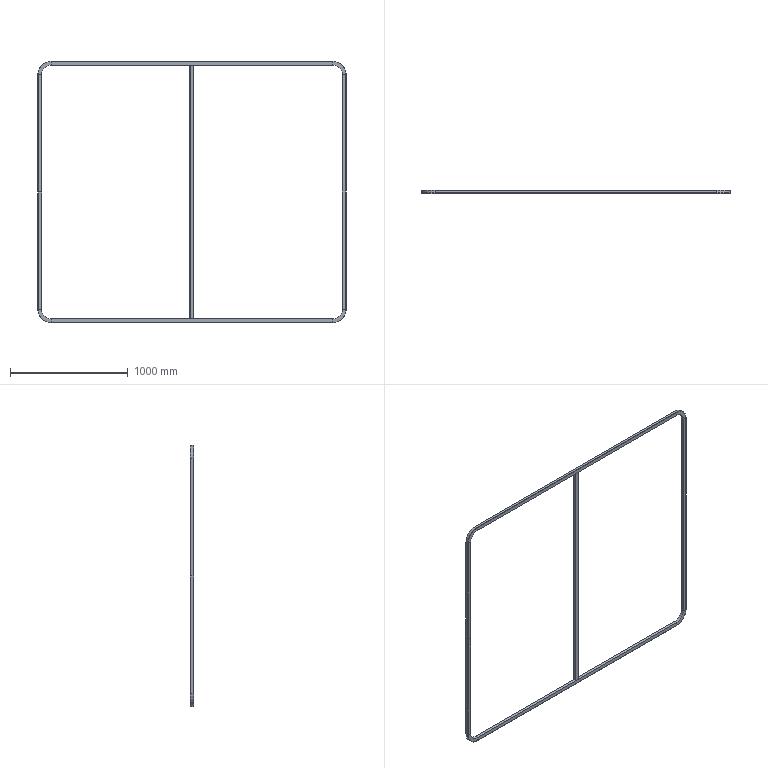Part | SolidWorks | features Fillet 1, ICE 1, Sweep 1 | 2 solids | 58 faces | box 2617 x 26 x 2217 mm | volume 9696679 mm3 | plane 34 | cylinder 16 | cone 4 | torus 4 | commonest cylinder face diameters 6 x12 160 x4
STEP:
#1=CARTESIAN_POINT('',(-1308.634,3.,995.));
#2=VERTEX_POINT('',#1);
#3=CARTESIAN_POINT('',(-1305.634,0.,995.));
#4=VERTEX_POINT('',#3);
#5=CARTESIAN_POINT('',(-1305.634,3.,995.));
#6=DIRECTION('',(0.,0.,1.));
#7=DIRECTION('',(-1.,0.,0.));
#8=AXIS2_PLACEMENT_3D('',#5,#6,#7);
#9=CIRCLE('',#8,3.);
#10=EDGE_CURVE('',#2,#4,#9,.T.);
#11=ORIENTED_EDGE('',*,*,#10,.F.);
#12=CARTESIAN_POINT('',(-1308.634,3.,0.));
#13=VERTEX_POINT('',#12);
#14=CARTESIAN_POINT('',(-1308.634,3.,995.));
#15=DIRECTION('',(0.,0.,-1.));
#16=VECTOR('',#15,1000.);
#17=LINE('',#14,#16);
#18=EDGE_CURVE('',#2,#13,#17,.T.);
#19=ORIENTED_EDGE('',*,*,#18,.T.);
#20=CARTESIAN_POINT('',(-1305.634,0.,0.));
#21=VERTEX_POINT('',#20);
#22=CARTESIAN_POINT('',(-1305.634,3.,0.));
#23=DIRECTION('',(0.,0.,1.));
#24=DIRECTION('',(-1.,0.,0.));
#25=AXIS2_PLACEMENT_3D('',#22,#23,#24);
#26=CIRCLE('',#25,3.);
#27=EDGE_CURVE('',#13,#21,#26,.T.);
#28=ORIENTED_EDGE('',*,*,#27,.T.);
#29=CARTESIAN_POINT('',(-1305.634,0.,995.));
#30=DIRECTION('',(0.,0.,-1.));
#31=VECTOR('',#30,1000.);
#32=LINE('',#29,#31);
#33=EDGE_CURVE('',#4,#21,#32,.T.);
#34=ORIENTED_EDGE('',*,*,#33,.F.);
#35=EDGE_LOOP('',(#11,#19,#28,#34));
#36=FACE_OUTER_BOUND('',#35,.T.);
#37=CARTESIAN_POINT('',(-1305.634,3.,995.));
#38=DIRECTION('',(0.,0.,-1.));
#39=DIRECTION('',(-1.,0.,0.));
#40=AXIS2_PLACEMENT_3D('',#37,#38,#39);
#41=CYLINDRICAL_SURFACE('',#40,3.);
#42=ADVANCED_FACE('',(#36),#41,.T.);
#43=CARTESIAN_POINT('',(1195.,3.,1108.634));
#44=VERTEX_POINT('',#43);
#45=CARTESIAN_POINT('',(1195.,0.,1105.634));
#46=VERTEX_POINT('',#45);
#47=CARTESIAN_POINT('',(1195.,3.,1105.634));
#48=DIRECTION('',(1.,0.,0.));
#49=DIRECTION('',(0.,0.,1.));
#50=AXIS2_PLACEMENT_3D('',#47,#48,#49);
#51=CIRCLE('',#50,3.);
#52=EDGE_CURVE('',#44,#46,#51,.T.);
#53=ORIENTED_EDGE('',*,*,#52,.F.);
#54=CARTESIAN_POINT('',(-1195.,3.,1108.634));
#55=VERTEX_POINT('',#54);
#56=CARTESIAN_POINT('',(1195.,3.,1108.634));
#57=DIRECTION('',(-1.,0.,0.));
#58=VECTOR('',#57,1000.);
#59=LINE('',#56,#58);
#60=EDGE_CURVE('',#44,#55,#59,.T.);
#61=ORIENTED_EDGE('',*,*,#60,.T.);
#62=CARTESIAN_POINT('',(-1195.,0.,1105.634));
#63=VERTEX_POINT('',#62);
#64=CARTESIAN_POINT('',(-1195.,3.,1105.634));
#65=DIRECTION('',(1.,0.,0.));
#66=DIRECTION('',(0.,0.,1.));
#67=AXIS2_PLACEMENT_3D('',#64,#65,#66);
#68=CIRCLE('',#67,3.);
#69=EDGE_CURVE('',#55,#63,#68,.T.);
#70=ORIENTED_EDGE('',*,*,#69,.T.);
#71=CARTESIAN_POINT('',(1195.,0.,1105.634));
#72=DIRECTION('',(-1.,0.,0.));
#73=VECTOR('',#72,1000.);
#74=LINE('',#71,#73);
#75=EDGE_CURVE('',#46,#63,#74,.T.);
#76=ORIENTED_EDGE('',*,*,#75,.F.);
#77=EDGE_LOOP('',(#53,#61,#70,#76));
#78=FACE_OUTER_BOUND('',#77,.T.);
#79=CARTESIAN_POINT('',(1195.,3.,1105.634));
#80=DIRECTION('',(-1.,0.,0.));
#81=DIRECTION('',(0.,0.,1.));
#82=AXIS2_PLACEMENT_3D('',#79,#80,#81);
#83=CYLINDRICAL_SURFACE('',#82,3.);
#84=ADVANCED_FACE('',(#78),#83,.T.);
#85=CARTESIAN_POINT('',(1308.634,3.,-995.));
#86=VERTEX_POINT('',#85);
#87=CARTESIAN_POINT('',(1305.634,0.,-995.));
#88=VERTEX_POINT('',#87);
#89=CARTESIAN_POINT('',(1305.634,3.,-995.));
#90=DIRECTION('',(0.,0.,-1.));
#91=DIRECTION('',(1.,0.,0.));
#92=AXIS2_PLACEMENT_3D('',#89,#90,#91);
#93=CIRCLE('',#92,3.);
#94=EDGE_CURVE('',#86,#88,#93,.T.);
#95=ORIENTED_EDGE('',*,*,#94,.F.);
#96=CARTESIAN_POINT('',(1308.634,3.,995.));
#97=VERTEX_POINT('',#96);
#98=CARTESIAN_POINT('',(1308.634,3.,-995.));
#99=DIRECTION('',(0.,0.,1.));
#100=VECTOR('',#99,1000.);
#101=LINE('',#98,#100);
#102=EDGE_CURVE('',#86,#97,#101,.T.);
#103=ORIENTED_EDGE('',*,*,#102,.T.);
#104=CARTESIAN_POINT('',(1305.634,0.,995.));
#105=VERTEX_POINT('',#104);
#106=CARTESIAN_POINT('',(1305.634,3.,995.));
#107=DIRECTION('',(0.,0.,-1.));
#108=DIRECTION('',(1.,0.,0.));
#109=AXIS2_PLACEMENT_3D('',#106,#107,#108);
#110=CIRCLE('',#109,3.);
#111=EDGE_CURVE('',#97,#105,#110,.T.);
#112=ORIENTED_EDGE('',*,*,#111,.T.);
#113=CARTESIAN_POINT('',(1305.634,0.,-995.));
#114=DIRECTION('',(0.,0.,1.));
#115=VECTOR('',#114,1000.);
#116=LINE('',#113,#115);
#117=EDGE_CURVE('',#88,#105,#116,.T.);
#118=ORIENTED_EDGE('',*,*,#117,.F.);
#119=EDGE_LOOP('',(#95,#103,#112,#118));
#120=FACE_OUTER_BOUND('',#119,.T.);
#121=CARTESIAN_POINT('',(1305.634,3.,-995.));
#122=DIRECTION('',(0.,0.,1.));
#123=DIRECTION('',(1.,0.,0.));
#124=AXIS2_PLACEMENT_3D('',#121,#122,#123);
#125=CYLINDRICAL_SURFACE('',#124,3.);
#126=ADVANCED_FACE('',(#120),#125,.T.);
#127=CARTESIAN_POINT('',(-1195.,3.,-1108.634));
#128=VERTEX_POINT('',#127);
#129=CARTESIAN_POINT('',(-1195.,0.,-1105.634));
#130=VERTEX_POINT('',#129);
#131=CARTESIAN_POINT('',(-1195.,3.,-1105.634));
#132=DIRECTION('',(-1.,0.,0.));
#133=DIRECTION('',(0.,0.,-1.));
#134=AXIS2_PLACEMENT_3D('',#131,#132,#133);
#135=CIRCLE('',#134,3.);
#136=EDGE_CURVE('',#128,#130,#135,.T.);
#137=ORIENTED_EDGE('',*,*,#136,.F.);
#138=CARTESIAN_POINT('',(1195.,3.,-1108.634));
#139=VERTEX_POINT('',#138);
#140=CARTESIAN_POINT('',(-1195.,3.,-1108.634));
#141=DIRECTION('',(1.,0.,0.));
#142=VECTOR('',#141,1000.);
#143=LINE('',#140,#142);
#144=EDGE_CURVE('',#128,#139,#143,.T.);
#145=ORIENTED_EDGE('',*,*,#144,.T.);
#146=CARTESIAN_POINT('',(1195.,0.,-1105.634));
#147=VERTEX_POINT('',#146);
#148=CARTESIAN_POINT('',(1195.,3.,-1105.634));
#149=DIRECTION('',(-1.,0.,0.));
#150=DIRECTION('',(0.,0.,-1.));
#151=AXIS2_PLACEMENT_3D('',#148,#149,#150);
#152=CIRCLE('',#151,3.);
#153=EDGE_CURVE('',#139,#147,#152,.T.);
#154=ORIENTED_EDGE('',*,*,#153,.T.);
#155=CARTESIAN_POINT('',(-1195.,0.,-1105.634));
#156=DIRECTION('',(1.,0.,0.));
#157=VECTOR('',#156,1000.);
#158=LINE('',#155,#157);
#159=EDGE_CURVE('',#130,#147,#158,.T.);
#160=ORIENTED_EDGE('',*,*,#159,.F.);
#161=EDGE_LOOP('',(#137,#145,#154,#160));
#162=FACE_OUTER_BOUND('',#161,.T.);
#163=CARTESIAN_POINT('',(-1195.,3.,-1105.634));
#164=DIRECTION('',(1.,0.,0.));
#165=DIRECTION('',(0.,0.,-1.));
#166=AXIS2_PLACEMENT_3D('',#163,#164,#165);
#167=CYLINDRICAL_SURFACE('',#166,3.);
#168=ADVANCED_FACE('',(#162),#167,.T.);
#169=ORIENTED_EDGE('',*,*,#27,.F.);
#170=CARTESIAN_POINT('',(-1308.634,3.,-995.));
#171=VERTEX_POINT('',#170);
#172=CARTESIAN_POINT('',(-1308.634,3.,0.));
#173=DIRECTION('',(0.,0.,-1.));
#174=VECTOR('',#173,1000.);
#175=LINE('',#172,#174);
#176=EDGE_CURVE('',#13,#171,#175,.T.);
#177=ORIENTED_EDGE('',*,*,#176,.T.);
#178=CARTESIAN_POINT('',(-1305.634,0.,-995.));
#179=VERTEX_POINT('',#178);
#180=CARTESIAN_POINT('',(-1305.634,3.,-995.));
#181=DIRECTION('',(0.,0.,1.));
#182=DIRECTION('',(-1.,0.,0.));
#183=AXIS2_PLACEMENT_3D('',#180,#181,#182);
#184=CIRCLE('',#183,3.);
#185=EDGE_CURVE('',#171,#179,#184,.T.);
#186=ORIENTED_EDGE('',*,*,#185,.T.);
#187=CARTESIAN_POINT('',(-1305.634,0.,0.));
#188=DIRECTION('',(0.,0.,-1.));
#189=VECTOR('',#188,1000.);
#190=LINE('',#187,#189);
#191=EDGE_CURVE('',#21,#179,#190,.T.);
#192=ORIENTED_EDGE('',*,*,#191,.F.);
#193=EDGE_LOOP('',(#169,#177,#186,#192));
#194=FACE_OUTER_BOUND('',#193,.T.);
#195=CARTESIAN_POINT('',(-1305.634,3.,0.));
#196=DIRECTION('',(0.,0.,-1.));
#197=DIRECTION('',(-1.,0.,0.));
#198=AXIS2_PLACEMENT_3D('',#195,#196,#197);
#199=CYLINDRICAL_SURFACE('',#198,3.);
#200=ADVANCED_FACE('',(#194),#199,.T.);
#201=CARTESIAN_POINT('',(-1306.,26.,995.));
#202=VERTEX_POINT('',#201);
#203=CARTESIAN_POINT('',(-1308.614,3.344,995.));
#204=VERTEX_POINT('',#203);
#205=CARTESIAN_POINT('',(-1308.614,3.344,995.));
#206=DIRECTION('',(-0.1146,-0.9934,0.));
#207=VECTOR('',#206,1000.);
#208=LINE('',#205,#207);
#209=EDGE_CURVE('',#202,#204,#208,.T.);
#210=ORIENTED_EDGE('',*,*,#209,.F.);
#211=CARTESIAN_POINT('',(-1306.,26.,0.));
#212=VERTEX_POINT('',#211);
#213=CARTESIAN_POINT('',(-1306.,26.,995.));
#214=DIRECTION('',(0.,0.,-1.));
#215=VECTOR('',#214,1000.);
#216=LINE('',#213,#215);
#217=EDGE_CURVE('',#202,#212,#216,.T.);
#218=ORIENTED_EDGE('',*,*,#217,.T.);
#219=CARTESIAN_POINT('',(-1308.614,3.344,0.));
#220=VERTEX_POINT('',#219);
#221=CARTESIAN_POINT('',(-1308.614,3.344,0.));
#222=DIRECTION('',(-0.1146,-0.9934,0.));
#223=VECTOR('',#222,1000.);
#224=LINE('',#221,#223);
#225=EDGE_CURVE('',#212,#220,#224,.T.);
#226=ORIENTED_EDGE('',*,*,#225,.T.);
#227=CARTESIAN_POINT('',(-1308.614,3.344,995.));
#228=DIRECTION('',(0.,0.,-1.));
#229=VECTOR('',#228,1000.);
#230=LINE('',#227,#229);
#231=EDGE_CURVE('',#204,#220,#230,.T.);
#232=ORIENTED_EDGE('',*,*,#231,.F.);
#233=EDGE_LOOP('',(#210,#218,#226,#232));
#234=FACE_OUTER_BOUND('',#233,.T.);
#235=CARTESIAN_POINT('',(-1308.614,3.344,995.));
#236=DIRECTION('',(0.9934,-0.1146,0.));
#237=DIRECTION('',(0.1146,0.9934,0.));
#238=AXIS2_PLACEMENT_3D('',#235,#236,#237);
#239=PLANE('',#238);
#240=ADVANCED_FACE('',(#234),#239,.F.);
#241=CARTESIAN_POINT('',(-1308.614,3.344,-995.));
#242=VERTEX_POINT('',#241);
#243=CARTESIAN_POINT('',(-1308.614,3.344,0.));
#244=DIRECTION('',(0.,0.,-1.));
#245=VECTOR('',#244,1000.);
#246=LINE('',#243,#245);
#247=EDGE_CURVE('',#220,#242,#246,.T.);
#248=ORIENTED_EDGE('',*,*,#247,.F.);
#249=ORIENTED_EDGE('',*,*,#225,.F.);
#250=CARTESIAN_POINT('',(-1306.,26.,-995.));
#251=VERTEX_POINT('',#250);
#252=CARTESIAN_POINT('',(-1306.,26.,0.));
#253=DIRECTION('',(0.,0.,-1.));
#254=VECTOR('',#253,1000.);
#255=LINE('',#252,#254);
#256=EDGE_CURVE('',#212,#251,#255,.T.);
#257=ORIENTED_EDGE('',*,*,#256,.T.);
#258=CARTESIAN_POINT('',(-1308.614,3.344,-995.));
#259=DIRECTION('',(-0.1146,-0.9934,0.));
#260=VECTOR('',#259,1000.);
#261=LINE('',#258,#260);
#262=EDGE_CURVE('',#251,#242,#261,.T.);
#263=ORIENTED_EDGE('',*,*,#262,.T.);
#264=EDGE_LOOP('',(#248,#249,#257,#263));
#265=FACE_OUTER_BOUND('',#264,.T.);
#266=CARTESIAN_POINT('',(-1308.614,3.344,0.));
#267=DIRECTION('',(0.9934,-0.1146,0.));
#268=DIRECTION('',(0.1146,0.9934,0.));
#269=AXIS2_PLACEMENT_3D('',#266,#267,#268);
#270=PLANE('',#269);
#271=ADVANCED_FACE('',(#265),#270,.F.);
#272=ORIENTED_EDGE('',*,*,#176,.F.);
#273=CARTESIAN_POINT('',(-1305.634,3.,0.));
#274=DIRECTION('',(0.,0.,1.));
#275=DIRECTION('',(-1.,0.,0.));
#276=AXIS2_PLACEMENT_3D('',#273,#274,#275);
#277=CIRCLE('',#276,3.);
#278=EDGE_CURVE('',#220,#13,#277,.T.);
#279=ORIENTED_EDGE('',*,*,#278,.F.);
#280=ORIENTED_EDGE('',*,*,#247,.T.);
#281=CARTESIAN_POINT('',(-1305.634,3.,-995.));
#282=DIRECTION('',(0.,0.,1.));
#283=DIRECTION('',(-1.,0.,0.));
#284=AXIS2_PLACEMENT_3D('',#281,#282,#283);
#285=CIRCLE('',#284,3.);
#286=EDGE_CURVE('',#242,#171,#285,.T.);
#287=ORIENTED_EDGE('',*,*,#286,.T.);
#288=EDGE_LOOP('',(#272,#279,#280,#287));
#289=FACE_OUTER_BOUND('',#288,.T.);
#290=CARTESIAN_POINT('',(-1305.634,3.,0.));
#291=DIRECTION('',(0.,0.,-1.));
#292=DIRECTION('',(-1.,0.,0.));
#293=AXIS2_PLACEMENT_3D('',#290,#291,#292);
#294=CYLINDRICAL_SURFACE('',#293,3.);
#295=ADVANCED_FACE('',(#289),#294,.T.);
#296=CARTESIAN_POINT('',(-1275.,0.,0.));
#297=VERTEX_POINT('',#296);
#298=CARTESIAN_POINT('',(-1275.,0.,-995.));
#299=VERTEX_POINT('',#298);
#300=CARTESIAN_POINT('',(-1275.,0.,0.));
#301=DIRECTION('',(0.,0.,-1.));
#302=VECTOR('',#301,1000.);
#303=LINE('',#300,#302);
#304=EDGE_CURVE('',#297,#299,#303,.T.);
#305=ORIENTED_EDGE('',*,*,#304,.F.);
#306=CARTESIAN_POINT('',(-1275.,0.,0.));
#307=DIRECTION('',(1.,0.,0.));
#308=VECTOR('',#307,1000.);
#309=LINE('',#306,#308);
#310=EDGE_CURVE('',#21,#297,#309,.T.);
#311=ORIENTED_EDGE('',*,*,#310,.F.);
#312=ORIENTED_EDGE('',*,*,#191,.T.);
#313=CARTESIAN_POINT('',(-1275.,0.,-995.));
#314=DIRECTION('',(1.,0.,0.));
#315=VECTOR('',#314,1000.);
#316=LINE('',#313,#315);
#317=EDGE_CURVE('',#179,#299,#316,.T.);
#318=ORIENTED_EDGE('',*,*,#317,.T.);
#319=EDGE_LOOP('',(#305,#311,#312,#318));
#320=FACE_OUTER_BOUND('',#319,.T.);
#321=CARTESIAN_POINT('',(-1275.,0.,0.));
#322=DIRECTION('',(0.,1.,0.));
#323=DIRECTION('',(-1.,0.,0.));
#324=AXIS2_PLACEMENT_3D('',#321,#322,#323);
#325=PLANE('',#324);
#326=ADVANCED_FACE('',(#320),#325,.F.);
#327=CARTESIAN_POINT('',(-1275.,26.,0.));
#328=VERTEX_POINT('',#327);
#329=CARTESIAN_POINT('',(-1275.,26.,-995.));
#330=VERTEX_POINT('',#329);
#331=CARTESIAN_POINT('',(-1275.,26.,0.));
#332=DIRECTION('',(0.,0.,-1.));
#333=VECTOR('',#332,1000.);
#334=LINE('',#331,#333);
#335=EDGE_CURVE('',#328,#330,#334,.T.);
#336=ORIENTED_EDGE('',*,*,#335,.F.);
#337=CARTESIAN_POINT('',(-1275.,26.,0.));
#338=DIRECTION('',(0.,1.,0.));
#339=VECTOR('',#338,1000.);
#340=LINE('',#337,#339);
#341=EDGE_CURVE('',#297,#328,#340,.T.);
#342=ORIENTED_EDGE('',*,*,#341,.F.);
#343=ORIENTED_EDGE('',*,*,#304,.T.);
#344=CARTESIAN_POINT('',(-1275.,26.,-995.));
#345=DIRECTION('',(0.,1.,0.));
#346=VECTOR('',#345,1000.);
#347=LINE('',#344,#346);
#348=EDGE_CURVE('',#299,#330,#347,.T.);
#349=ORIENTED_EDGE('',*,*,#348,.T.);
#350=EDGE_LOOP('',(#336,#342,#343,#349));
#351=FACE_OUTER_BOUND('',#350,.T.);
#352=CARTESIAN_POINT('',(-1275.,26.,0.));
#353=DIRECTION('',(-1.,0.,0.));
#354=DIRECTION('',(0.,0.,1.));
#355=AXIS2_PLACEMENT_3D('',#352,#353,#354);
#356=PLANE('',#355);
#357=ADVANCED_FACE('',(#351),#356,.F.);
#358=CARTESIAN_POINT('',(-1306.,26.,-995.));
#359=DIRECTION('',(-1.,0.,0.));
#360=VECTOR('',#359,1000.);
#361=LINE('',#358,#360);
#362=EDGE_CURVE('',#330,#251,#361,.T.);
#363=ORIENTED_EDGE('',*,*,#362,.T.);
#364=ORIENTED_EDGE('',*,*,#256,.F.);
#365=CARTESIAN_POINT('',(-1306.,26.,0.));
#366=DIRECTION('',(-1.,0.,0.));
#367=VECTOR('',#366,1000.);
#368=LINE('',#365,#367);
#369=EDGE_CURVE('',#328,#212,#368,.T.);
#370=ORIENTED_EDGE('',*,*,#369,.F.);
#371=ORIENTED_EDGE('',*,*,#335,.T.);
#372=EDGE_LOOP('',(#363,#364,#370,#371));
#373=FACE_OUTER_BOUND('',#372,.T.);
#374=CARTESIAN_POINT('',(-1306.,26.,0.));
#375=DIRECTION('',(0.,-1.,0.));
#376=DIRECTION('',(0.,0.,-1.));
#377=AXIS2_PLACEMENT_3D('',#374,#375,#376);
#378=PLANE('',#377);
#379=ADVANCED_FACE('',(#373),#378,.F.);
#380=CARTESIAN_POINT('',(-1195.,3.344,-1108.614));
#381=VERTEX_POINT('',#380);
#382=CARTESIAN_POINT('',(-1195.,3.344,-995.));
#383=DIRECTION('',(0.,-1.,0.));
#384=DIRECTION('',(-1.,0.,0.));
#385=AXIS2_PLACEMENT_3D('',#382,#383,#384);
#386=CIRCLE('',#385,113.614);
#387=EDGE_CURVE('',#242,#381,#386,.T.);
#388=ORIENTED_EDGE('',*,*,#387,.F.);
#389=ORIENTED_EDGE('',*,*,#262,.F.);
#390=CARTESIAN_POINT('',(-1195.,26.,-1106.));
#391=VERTEX_POINT('',#390);
#392=CARTESIAN_POINT('',(-1195.,26.,-995.));
#393=DIRECTION('',(0.,-1.,0.));
#394=DIRECTION('',(-1.,0.,0.));
#395=AXIS2_PLACEMENT_3D('',#392,#393,#394);
#396=CIRCLE('',#395,111.);
#397=EDGE_CURVE('',#251,#391,#396,.T.);
#398=ORIENTED_EDGE('',*,*,#397,.T.);
#399=CARTESIAN_POINT('',(-1195.,3.344,-1108.614));
#400=DIRECTION('',(0.,-0.9934,-0.1146));
#401=VECTOR('',#400,1000.);
#402=LINE('',#399,#401);
#403=EDGE_CURVE('',#391,#381,#402,.T.);
#404=ORIENTED_EDGE('',*,*,#403,.T.);
#405=EDGE_LOOP('',(#388,#389,#398,#404));
#406=FACE_OUTER_BOUND('',#405,.T.);
#407=CARTESIAN_POINT('',(-1195.,26.,-995.));
#408=DIRECTION('',(0.,-1.,0.));
#409=DIRECTION('',(0.,0.,-1.));
#410=AXIS2_PLACEMENT_3D('',#407,#408,#409);
#411=CONICAL_SURFACE('',#410,111.,0.1149);
#412=ADVANCED_FACE('',(#406),#411,.T.);
#413=CARTESIAN_POINT('',(-1195.,0.,-995.));
#414=DIRECTION('',(0.,-1.,0.));
#415=DIRECTION('',(-1.,0.,0.));
#416=AXIS2_PLACEMENT_3D('',#413,#414,#415);
#417=CIRCLE('',#416,110.634);
#418=EDGE_CURVE('',#179,#130,#417,.T.);
#419=ORIENTED_EDGE('',*,*,#418,.F.);
#420=ORIENTED_EDGE('',*,*,#185,.F.);
#421=ORIENTED_EDGE('',*,*,#286,.F.);
#422=ORIENTED_EDGE('',*,*,#387,.T.);
#423=CARTESIAN_POINT('',(-1195.,3.,-1105.634));
#424=DIRECTION('',(-1.,0.,0.));
#425=DIRECTION('',(0.,0.,-1.));
#426=AXIS2_PLACEMENT_3D('',#423,#424,#425);
#427=CIRCLE('',#426,3.);
#428=EDGE_CURVE('',#381,#128,#427,.T.);
#429=ORIENTED_EDGE('',*,*,#428,.T.);
#430=ORIENTED_EDGE('',*,*,#136,.T.);
#431=EDGE_LOOP('',(#419,#420,#421,#422,#429,#430));
#432=FACE_OUTER_BOUND('',#431,.T.);
#433=CARTESIAN_POINT('',(-1195.,3.,-995.));
#434=DIRECTION('',(0.,-1.,0.));
#435=DIRECTION('',(0.,0.,-1.));
#436=AXIS2_PLACEMENT_3D('',#433,#434,#435);
#437=TOROIDAL_SURFACE('',#436,110.634,3.);
#438=ADVANCED_FACE('',(#432),#437,.T.);
#439=CARTESIAN_POINT('',(-1195.,0.,-1075.));
#440=VERTEX_POINT('',#439);
#441=CARTESIAN_POINT('',(-1195.,0.,-995.));
#442=DIRECTION('',(0.,-1.,0.));
#443=DIRECTION('',(-1.,0.,0.));
#444=AXIS2_PLACEMENT_3D('',#441,#442,#443);
#445=CIRCLE('',#444,80.);
#446=EDGE_CURVE('',#299,#440,#445,.T.);
#447=ORIENTED_EDGE('',*,*,#446,.F.);
#448=ORIENTED_EDGE('',*,*,#317,.F.);
#449=ORIENTED_EDGE('',*,*,#418,.T.);
#450=CARTESIAN_POINT('',(-1195.,0.,-1075.));
#451=DIRECTION('',(0.,0.,1.));
#452=VECTOR('',#451,1000.);
#453=LINE('',#450,#452);
#454=EDGE_CURVE('',#130,#440,#453,.T.);
#455=ORIENTED_EDGE('',*,*,#454,.T.);
#456=EDGE_LOOP('',(#447,#448,#449,#455));
#457=FACE_OUTER_BOUND('',#456,.T.);
#458=CARTESIAN_POINT('',(-1275.,0.,-995.));
#459=DIRECTION('',(0.,1.,0.));
#460=DIRECTION('',(0.,0.,1.));
#461=AXIS2_PLACEMENT_3D('',#458,#459,#460);
#462=PLANE('',#461);
#463=ADVANCED_FACE('',(#457),#462,.F.);
#464=CARTESIAN_POINT('',(-1195.,26.,-1075.));
#465=VERTEX_POINT('',#464);
#466=CARTESIAN_POINT('',(-1195.,26.,-995.));
#467=DIRECTION('',(0.,-1.,0.));
#468=DIRECTION('',(-1.,0.,0.));
#469=AXIS2_PLACEMENT_3D('',#466,#467,#468);
#470=CIRCLE('',#469,80.);
#471=EDGE_CURVE('',#330,#465,#470,.T.);
#472=ORIENTED_EDGE('',*,*,#471,.F.);
#473=ORIENTED_EDGE('',*,*,#348,.F.);
#474=ORIENTED_EDGE('',*,*,#446,.T.);
#475=CARTESIAN_POINT('',(-1195.,26.,-1075.));
#476=DIRECTION('',(0.,1.,0.));
#477=VECTOR('',#476,1000.);
#478=LINE('',#475,#477);
#479=EDGE_CURVE('',#440,#465,#478,.T.);
#480=ORIENTED_EDGE('',*,*,#479,.T.);
#481=EDGE_LOOP('',(#472,#473,#474,#480));
#482=FACE_OUTER_BOUND('',#481,.T.);
#483=CARTESIAN_POINT('',(-1195.,0.,-995.));
#484=DIRECTION('',(0.,-1.,0.));
#485=DIRECTION('',(0.,0.,-1.));
#486=AXIS2_PLACEMENT_3D('',#483,#484,#485);
#487=CYLINDRICAL_SURFACE('',#486,80.);
#488=ADVANCED_FACE('',(#482),#487,.F.);
#489=CARTESIAN_POINT('',(-1195.,26.,-1106.));
#490=DIRECTION('',(0.,0.,-1.));
#491=VECTOR('',#490,1000.);
#492=LINE('',#489,#491);
#493=EDGE_CURVE('',#465,#391,#492,.T.);
#494=ORIENTED_EDGE('',*,*,#493,.T.);
#495=ORIENTED_EDGE('',*,*,#397,.F.);
#496=ORIENTED_EDGE('',*,*,#362,.F.);
#497=ORIENTED_EDGE('',*,*,#471,.T.);
#498=EDGE_LOOP('',(#494,#495,#496,#497));
#499=FACE_OUTER_BOUND('',#498,.T.);
#500=CARTESIAN_POINT('',(-1306.,26.,-995.));
#501=DIRECTION('',(0.,-1.,0.));
#502=DIRECTION('',(0.,0.,-1.));
#503=AXIS2_PLACEMENT_3D('',#500,#501,#502);
#504=PLANE('',#503);
#505=ADVANCED_FACE('',(#499),#504,.F.);
#506=CARTESIAN_POINT('',(1195.,3.344,-1108.614));
#507=VERTEX_POINT('',#506);
#508=CARTESIAN_POINT('',(-1195.,3.344,-1108.614));
#509=DIRECTION('',(1.,0.,0.));
#510=VECTOR('',#509,1000.);
#511=LINE('',#508,#510);
#512=EDGE_CURVE('',#381,#507,#511,.T.);
#513=ORIENTED_EDGE('',*,*,#512,.F.);
#514=ORIENTED_EDGE('',*,*,#403,.F.);
#515=CARTESIAN_POINT('',(1195.,26.,-1106.));
#516=VERTEX_POINT('',#515);
#517=CARTESIAN_POINT('',(-1195.,26.,-1106.));
#518=DIRECTION('',(1.,0.,0.));
#519=VECTOR('',#518,1000.);
#520=LINE('',#517,#519);
#521=EDGE_CURVE('',#391,#516,#520,.T.);
#522=ORIENTED_EDGE('',*,*,#521,.T.);
#523=CARTESIAN_POINT('',(1195.,3.344,-1108.614));
#524=DIRECTION('',(0.,-0.9934,-0.1146));
#525=VECTOR('',#524,1000.);
#526=LINE('',#523,#525);
#527=EDGE_CURVE('',#516,#507,#526,.T.);
#528=ORIENTED_EDGE('',*,*,#527,.T.);
#529=EDGE_LOOP('',(#513,#514,#522,#528));
#530=FACE_OUTER_BOUND('',#529,.T.);
#531=CARTESIAN_POINT('',(-1195.,3.344,-1108.614));
#532=DIRECTION('',(0.,-0.1146,0.9934));
#533=DIRECTION('',(0.,-0.9934,-0.1146));
#534=AXIS2_PLACEMENT_3D('',#531,#532,#533);
#535=PLANE('',#534);
#536=ADVANCED_FACE('',(#530),#535,.F.);
#537=ORIENTED_EDGE('',*,*,#144,.F.);
#538=ORIENTED_EDGE('',*,*,#428,.F.);
#539=ORIENTED_EDGE('',*,*,#512,.T.);
#540=CARTESIAN_POINT('',(1195.,3.,-1105.634));
#541=DIRECTION('',(-1.,0.,0.));
#542=DIRECTION('',(0.,0.,-1.));
#543=AXIS2_PLACEMENT_3D('',#540,#541,#542);
#544=CIRCLE('',#543,3.);
#545=EDGE_CURVE('',#507,#139,#544,.T.);
#546=ORIENTED_EDGE('',*,*,#545,.T.);
#547=EDGE_LOOP('',(#537,#538,#539,#546));
#548=FACE_OUTER_BOUND('',#547,.T.);
#549=CARTESIAN_POINT('',(-1195.,3.,-1105.634));
#550=DIRECTION('',(1.,0.,0.));
#551=DIRECTION('',(0.,0.,-1.));
#552=AXIS2_PLACEMENT_3D('',#549,#550,#551);
#553=CYLINDRICAL_SURFACE('',#552,3.);
#554=ADVANCED_FACE('',(#548),#553,.T.);
#555=CARTESIAN_POINT('',(1195.,0.,-1075.));
#556=VERTEX_POINT('',#555);
#557=CARTESIAN_POINT('',(-1195.,0.,-1075.));
#558=DIRECTION('',(1.,0.,0.));
#559=VECTOR('',#558,1000.);
#560=LINE('',#557,#559);
#561=EDGE_CURVE('',#440,#556,#560,.T.);
#562=ORIENTED_EDGE('',*,*,#561,.F.);
#563=ORIENTED_EDGE('',*,*,#454,.F.);
#564=ORIENTED_EDGE('',*,*,#159,.T.);
#565=CARTESIAN_POINT('',(1195.,0.,-1075.));
#566=DIRECTION('',(0.,0.,1.));
#567=VECTOR('',#566,1000.);
#568=LINE('',#565,#567);
#569=EDGE_CURVE('',#147,#556,#568,.T.);
#570=ORIENTED_EDGE('',*,*,#569,.T.);
#571=EDGE_LOOP('',(#562,#563,#564,#570));
#572=FACE_OUTER_BOUND('',#571,.T.);
#573=CARTESIAN_POINT('',(-1195.,0.,-1075.));
#574=DIRECTION('',(0.,1.,0.));
#575=DIRECTION('',(0.,0.,1.));
#576=AXIS2_PLACEMENT_3D('',#573,#574,#575);
#577=PLANE('',#576);
#578=ADVANCED_FACE('',(#572),#577,.F.);
#579=CARTESIAN_POINT('',(1195.,26.,-1075.));
#580=VERTEX_POINT('',#579);
#581=CARTESIAN_POINT('',(-1195.,26.,-1075.));
#582=DIRECTION('',(1.,0.,0.));
#583=VECTOR('',#582,1000.);
#584=LINE('',#581,#583);
#585=EDGE_CURVE('',#465,#580,#584,.T.);
#586=ORIENTED_EDGE('',*,*,#585,.F.);
#587=ORIENTED_EDGE('',*,*,#479,.F.);
#588=ORIENTED_EDGE('',*,*,#561,.T.);
#589=CARTESIAN_POINT('',(1195.,26.,-1075.));
#590=DIRECTION('',(0.,1.,0.));
#591=VECTOR('',#590,1000.);
#592=LINE('',#589,#591);
#593=EDGE_CURVE('',#556,#580,#592,.T.);
#594=ORIENTED_EDGE('',*,*,#593,.T.);
#595=EDGE_LOOP('',(#586,#587,#588,#594));
#596=FACE_OUTER_BOUND('',#595,.T.);
#597=CARTESIAN_POINT('',(-1195.,26.,-1075.));
#598=DIRECTION('',(0.,0.,-1.));
#599=DIRECTION('',(-1.,0.,0.));
#600=AXIS2_PLACEMENT_3D('',#597,#598,#599);
#601=PLANE('',#600);
#602=ADVANCED_FACE('',(#596),#601,.F.);
#603=CARTESIAN_POINT('',(1195.,26.,-1106.));
#604=DIRECTION('',(0.,0.,-1.));
#605=VECTOR('',#604,1000.);
#606=LINE('',#603,#605);
#607=EDGE_CURVE('',#580,#516,#606,.T.);
#608=ORIENTED_EDGE('',*,*,#607,.T.);
#609=ORIENTED_EDGE('',*,*,#521,.F.);
#610=ORIENTED_EDGE('',*,*,#493,.F.);
#611=ORIENTED_EDGE('',*,*,#585,.T.);
#612=EDGE_LOOP('',(#608,#609,#610,#611));
#613=FACE_OUTER_BOUND('',#612,.T.);
#614=CARTESIAN_POINT('',(-1195.,26.,-1106.));
#615=DIRECTION('',(0.,-1.,0.));
#616=DIRECTION('',(0.,0.,-1.));
#617=AXIS2_PLACEMENT_3D('',#614,#615,#616);
#618=PLANE('',#617);
#619=ADVANCED_FACE('',(#613),#618,.F.);
#620=CARTESIAN_POINT('',(1308.614,3.344,-995.));
#621=VERTEX_POINT('',#620);
#622=CARTESIAN_POINT('',(1195.,3.344,-995.));
#623=DIRECTION('',(0.,-1.,0.));
#624=DIRECTION('',(0.,0.,-1.));
#625=AXIS2_PLACEMENT_3D('',#622,#623,#624);
#626=CIRCLE('',#625,113.614);
#627=EDGE_CURVE('',#507,#621,#626,.T.);
#628=ORIENTED_EDGE('',*,*,#627,.F.);
#629=ORIENTED_EDGE('',*,*,#527,.F.);
#630=CARTESIAN_POINT('',(1306.,26.,-995.));
#631=VERTEX_POINT('',#630);
#632=CARTESIAN_POINT('',(1195.,26.,-995.));
#633=DIRECTION('',(0.,-1.,0.));
#634=DIRECTION('',(0.,0.,-1.));
#635=AXIS2_PLACEMENT_3D('',#632,#633,#634);
#636=CIRCLE('',#635,111.);
#637=EDGE_CURVE('',#516,#631,#636,.T.);
#638=ORIENTED_EDGE('',*,*,#637,.T.);
#639=CARTESIAN_POINT('',(1308.614,3.344,-995.));
#640=DIRECTION('',(0.1146,-0.9934,0.));
#641=VECTOR('',#640,1000.);
#642=LINE('',#639,#641);
#643=EDGE_CURVE('',#631,#621,#642,.T.);
#644=ORIENTED_EDGE('',*,*,#643,.T.);
#645=EDGE_LOOP('',(#628,#629,#638,#644));
#646=FACE_OUTER_BOUND('',#645,.T.);
#647=CARTESIAN_POINT('',(1195.,26.,-995.));
#648=DIRECTION('',(0.,-1.,0.));
#649=DIRECTION('',(0.,0.,-1.));
#650=AXIS2_PLACEMENT_3D('',#647,#648,#649);
#651=CONICAL_SURFACE('',#650,111.,0.1149);
#652=ADVANCED_FACE('',(#646),#651,.T.);
#653=CARTESIAN_POINT('',(1195.,0.,-995.));
#654=DIRECTION('',(0.,-1.,0.));
#655=DIRECTION('',(0.,0.,-1.));
#656=AXIS2_PLACEMENT_3D('',#653,#654,#655);
#657=CIRCLE('',#656,110.634);
#658=EDGE_CURVE('',#147,#88,#657,.T.);
#659=ORIENTED_EDGE('',*,*,#658,.F.);
#660=ORIENTED_EDGE('',*,*,#153,.F.);
#661=ORIENTED_EDGE('',*,*,#545,.F.);
#662=ORIENTED_EDGE('',*,*,#627,.T.);
#663=CARTESIAN_POINT('',(1305.634,3.,-995.));
#664=DIRECTION('',(0.,0.,-1.));
#665=DIRECTION('',(1.,0.,0.));
#666=AXIS2_PLACEMENT_3D('',#663,#664,#665);
#667=CIRCLE('',#666,3.);
#668=EDGE_CURVE('',#621,#86,#667,.T.);
#669=ORIENTED_EDGE('',*,*,#668,.T.);
#670=ORIENTED_EDGE('',*,*,#94,.T.);
#671=EDGE_LOOP('',(#659,#660,#661,#662,#669,#670));
#672=FACE_OUTER_BOUND('',#671,.T.);
#673=CARTESIAN_POINT('',(1195.,3.,-995.));
#674=DIRECTION('',(0.,-1.,0.));
#675=DIRECTION('',(0.,0.,-1.));
#676=AXIS2_PLACEMENT_3D('',#673,#674,#675);
#677=TOROIDAL_SURFACE('',#676,110.634,3.);
#678=ADVANCED_FACE('',(#672),#677,.T.);
#679=CARTESIAN_POINT('',(1275.,0.,-995.));
#680=VERTEX_POINT('',#679);
#681=CARTESIAN_POINT('',(1195.,0.,-995.));
#682=DIRECTION('',(0.,-1.,0.));
#683=DIRECTION('',(0.,0.,-1.));
#684=AXIS2_PLACEMENT_3D('',#681,#682,#683);
#685=CIRCLE('',#684,80.);
#686=EDGE_CURVE('',#556,#680,#685,.T.);
#687=ORIENTED_EDGE('',*,*,#686,.F.);
#688=ORIENTED_EDGE('',*,*,#569,.F.);
#689=ORIENTED_EDGE('',*,*,#658,.T.);
#690=CARTESIAN_POINT('',(1275.,0.,-995.));
#691=DIRECTION('',(-1.,0.,0.));
#692=VECTOR('',#691,1000.);
#693=LINE('',#690,#692);
#694=EDGE_CURVE('',#88,#680,#693,.T.);
#695=ORIENTED_EDGE('',*,*,#694,.T.);
#696=EDGE_LOOP('',(#687,#688,#689,#695));
#697=FACE_OUTER_BOUND('',#696,.T.);
#698=CARTESIAN_POINT('',(1195.,0.,-1075.));
#699=DIRECTION('',(0.,1.,0.));
#700=DIRECTION('',(0.,0.,1.));
#701=AXIS2_PLACEMENT_3D('',#698,#699,#700);
#702=PLANE('',#701);
#703=ADVANCED_FACE('',(#697),#702,.F.);
#704=CARTESIAN_POINT('',(1275.,26.,-995.));
#705=VERTEX_POINT('',#704);
#706=CARTESIAN_POINT('',(1195.,26.,-995.));
#707=DIRECTION('',(0.,-1.,0.));
#708=DIRECTION('',(0.,0.,-1.));
#709=AXIS2_PLACEMENT_3D('',#706,#707,#708);
#710=CIRCLE('',#709,80.);
#711=EDGE_CURVE('',#580,#705,#710,.T.);
#712=ORIENTED_EDGE('',*,*,#711,.F.);
#713=ORIENTED_EDGE('',*,*,#593,.F.);
#714=ORIENTED_EDGE('',*,*,#686,.T.);
#715=CARTESIAN_POINT('',(1275.,26.,-995.));
#716=DIRECTION('',(0.,1.,0.));
#717=VECTOR('',#716,1000.);
#718=LINE('',#715,#717);
#719=EDGE_CURVE('',#680,#705,#718,.T.);
#720=ORIENTED_EDGE('',*,*,#719,.T.);
#721=EDGE_LOOP('',(#712,#713,#714,#720));
#722=FACE_OUTER_BOUND('',#721,.T.);
#723=CARTESIAN_POINT('',(1195.,0.,-995.));
#724=DIRECTION('',(0.,-1.,0.));
#725=DIRECTION('',(0.,0.,-1.));
#726=AXIS2_PLACEMENT_3D('',#723,#724,#725);
#727=CYLINDRICAL_SURFACE('',#726,80.);
#728=ADVANCED_FACE('',(#722),#727,.F.);
#729=CARTESIAN_POINT('',(1306.,26.,-995.));
#730=DIRECTION('',(1.,0.,0.));
#731=VECTOR('',#730,1000.);
#732=LINE('',#729,#731);
#733=EDGE_CURVE('',#705,#631,#732,.T.);
#734=ORIENTED_EDGE('',*,*,#733,.T.);
#735=ORIENTED_EDGE('',*,*,#637,.F.);
#736=ORIENTED_EDGE('',*,*,#607,.F.);
#737=ORIENTED_EDGE('',*,*,#711,.T.);
#738=EDGE_LOOP('',(#734,#735,#736,#737));
#739=FACE_OUTER_BOUND('',#738,.T.);
#740=CARTESIAN_POINT('',(1195.,26.,-1106.));
#741=DIRECTION('',(0.,-1.,0.));
#742=DIRECTION('',(0.,0.,-1.));
#743=AXIS2_PLACEMENT_3D('',#740,#741,#742);
#744=PLANE('',#743);
#745=ADVANCED_FACE('',(#739),#744,.F.);
#746=CARTESIAN_POINT('',(1308.614,3.344,995.));
#747=VERTEX_POINT('',#746);
#748=CARTESIAN_POINT('',(1308.614,3.344,-995.));
#749=DIRECTION('',(0.,0.,1.));
#750=VECTOR('',#749,1000.);
#751=LINE('',#748,#750);
#752=EDGE_CURVE('',#621,#747,#751,.T.);
#753=ORIENTED_EDGE('',*,*,#752,.F.);
#754=ORIENTED_EDGE('',*,*,#643,.F.);
#755=CARTESIAN_POINT('',(1306.,26.,995.));
#756=VERTEX_POINT('',#755);
#757=CARTESIAN_POINT('',(1306.,26.,-995.));
#758=DIRECTION('',(0.,0.,1.));
#759=VECTOR('',#758,1000.);
#760=LINE('',#757,#759);
#761=EDGE_CURVE('',#631,#756,#760,.T.);
#762=ORIENTED_EDGE('',*,*,#761,.T.);
#763=CARTESIAN_POINT('',(1308.614,3.344,995.));
#764=DIRECTION('',(0.1146,-0.9934,0.));
#765=VECTOR('',#764,1000.);
#766=LINE('',#763,#765);
#767=EDGE_CURVE('',#756,#747,#766,.T.);
#768=ORIENTED_EDGE('',*,*,#767,.T.);
#769=EDGE_LOOP('',(#753,#754,#762,#768));
#770=FACE_OUTER_BOUND('',#769,.T.);
#771=CARTESIAN_POINT('',(1308.614,3.344,-995.));
#772=DIRECTION('',(-0.9934,-0.1146,0.));
#773=DIRECTION('',(0.1146,-0.9934,0.));
#774=AXIS2_PLACEMENT_3D('',#771,#772,#773);
#775=PLANE('',#774);
#776=ADVANCED_FACE('',(#770),#775,.F.);
#777=ORIENTED_EDGE('',*,*,#102,.F.);
#778=ORIENTED_EDGE('',*,*,#668,.F.);
#779=ORIENTED_EDGE('',*,*,#752,.T.);
#780=CARTESIAN_POINT('',(1305.634,3.,995.));
#781=DIRECTION('',(0.,0.,-1.));
#782=DIRECTION('',(1.,0.,0.));
#783=AXIS2_PLACEMENT_3D('',#780,#781,#782);
#784=CIRCLE('',#783,3.);
#785=EDGE_CURVE('',#747,#97,#784,.T.);
#786=ORIENTED_EDGE('',*,*,#785,.T.);
#787=EDGE_LOOP('',(#777,#778,#779,#786));
#788=FACE_OUTER_BOUND('',#787,.T.);
#789=CARTESIAN_POINT('',(1305.634,3.,-995.));
#790=DIRECTION('',(0.,0.,1.));
#791=DIRECTION('',(1.,0.,0.));
#792=AXIS2_PLACEMENT_3D('',#789,#790,#791);
#793=CYLINDRICAL_SURFACE('',#792,3.);
#794=ADVANCED_FACE('',(#788),#793,.T.);
#795=CARTESIAN_POINT('',(1275.,0.,995.));
#796=VERTEX_POINT('',#795);
#797=CARTESIAN_POINT('',(1275.,0.,-995.));
#798=DIRECTION('',(0.,0.,1.));
#799=VECTOR('',#798,1000.);
#800=LINE('',#797,#799);
#801=EDGE_CURVE('',#680,#796,#800,.T.);
#802=ORIENTED_EDGE('',*,*,#801,.F.);
#803=ORIENTED_EDGE('',*,*,#694,.F.);
#804=ORIENTED_EDGE('',*,*,#117,.T.);
#805=CARTESIAN_POINT('',(1275.,0.,995.));
#806=DIRECTION('',(-1.,0.,0.));
#807=VECTOR('',#806,1000.);
#808=LINE('',#805,#807);
#809=EDGE_CURVE('',#105,#796,#808,.T.);
#810=ORIENTED_EDGE('',*,*,#809,.T.);
#811=EDGE_LOOP('',(#802,#803,#804,#810));
#812=FACE_OUTER_BOUND('',#811,.T.);
#813=CARTESIAN_POINT('',(1275.,0.,-995.));
#814=DIRECTION('',(0.,1.,0.));
#815=DIRECTION('',(-1.,0.,0.));
#816=AXIS2_PLACEMENT_3D('',#813,#814,#815);
#817=PLANE('',#816);
#818=ADVANCED_FACE('',(#812),#817,.F.);
#819=CARTESIAN_POINT('',(1275.,26.,995.));
#820=VERTEX_POINT('',#819);
#821=CARTESIAN_POINT('',(1275.,26.,-995.));
#822=DIRECTION('',(0.,0.,1.));
#823=VECTOR('',#822,1000.);
#824=LINE('',#821,#823);
#825=EDGE_CURVE('',#705,#820,#824,.T.);
#826=ORIENTED_EDGE('',*,*,#825,.F.);
#827=ORIENTED_EDGE('',*,*,#719,.F.);
#828=ORIENTED_EDGE('',*,*,#801,.T.);
#829=CARTESIAN_POINT('',(1275.,26.,995.));
#830=DIRECTION('',(0.,1.,0.));
#831=VECTOR('',#830,1000.);
#832=LINE('',#829,#831);
#833=EDGE_CURVE('',#796,#820,#832,.T.);
#834=ORIENTED_EDGE('',*,*,#833,.T.);
#835=EDGE_LOOP('',(#826,#827,#828,#834));
#836=FACE_OUTER_BOUND('',#835,.T.);
#837=CARTESIAN_POINT('',(1275.,26.,-995.));
#838=DIRECTION('',(1.,0.,0.));
#839=DIRECTION('',(0.,0.,-1.));
#840=AXIS2_PLACEMENT_3D('',#837,#838,#839);
#841=PLANE('',#840);
#842=ADVANCED_FACE('',(#836),#841,.F.);
#843=CARTESIAN_POINT('',(1306.,26.,995.));
#844=DIRECTION('',(1.,0.,0.));
#845=VECTOR('',#844,1000.);
#846=LINE('',#843,#845);
#847=EDGE_CURVE('',#820,#756,#846,.T.);
#848=ORIENTED_EDGE('',*,*,#847,.T.);
#849=ORIENTED_EDGE('',*,*,#761,.F.);
#850=ORIENTED_EDGE('',*,*,#733,.F.);
#851=ORIENTED_EDGE('',*,*,#825,.T.);
#852=EDGE_LOOP('',(#848,#849,#850,#851));
#853=FACE_OUTER_BOUND('',#852,.T.);
#854=CARTESIAN_POINT('',(1306.,26.,-995.));
#855=DIRECTION('',(0.,-1.,0.));
#856=DIRECTION('',(0.,0.,-1.));
#857=AXIS2_PLACEMENT_3D('',#854,#855,#856);
#858=PLANE('',#857);
#859=ADVANCED_FACE('',(#853),#858,.F.);
#860=CARTESIAN_POINT('',(1195.,3.344,1108.614));
#861=VERTEX_POINT('',#860);
#862=CARTESIAN_POINT('',(1195.,3.344,995.));
#863=DIRECTION('',(0.,-1.,0.));
#864=DIRECTION('',(1.,0.,0.));
#865=AXIS2_PLACEMENT_3D('',#862,#863,#864);
#866=CIRCLE('',#865,113.614);
#867=EDGE_CURVE('',#747,#861,#866,.T.);
#868=ORIENTED_EDGE('',*,*,#867,.F.);
#869=ORIENTED_EDGE('',*,*,#767,.F.);
#870=CARTESIAN_POINT('',(1195.,26.,1106.));
#871=VERTEX_POINT('',#870);
#872=CARTESIAN_POINT('',(1195.,26.,995.));
#873=DIRECTION('',(0.,-1.,0.));
#874=DIRECTION('',(1.,0.,0.));
#875=AXIS2_PLACEMENT_3D('',#872,#873,#874);
#876=CIRCLE('',#875,111.);
#877=EDGE_CURVE('',#756,#871,#876,.T.);
#878=ORIENTED_EDGE('',*,*,#877,.T.);
#879=CARTESIAN_POINT('',(1195.,3.344,1108.614));
#880=DIRECTION('',(0.,-0.9934,0.1146));
#881=VECTOR('',#880,1000.);
#882=LINE('',#879,#881);
#883=EDGE_CURVE('',#871,#861,#882,.T.);
#884=ORIENTED_EDGE('',*,*,#883,.T.);
#885=EDGE_LOOP('',(#868,#869,#878,#884));
#886=FACE_OUTER_BOUND('',#885,.T.);
#887=CARTESIAN_POINT('',(1195.,26.,995.));
#888=DIRECTION('',(0.,-1.,0.));
#889=DIRECTION('',(0.,0.,-1.));
#890=AXIS2_PLACEMENT_3D('',#887,#888,#889);
#891=CONICAL_SURFACE('',#890,111.,0.1149);
#892=ADVANCED_FACE('',(#886),#891,.T.);
#893=CARTESIAN_POINT('',(1195.,0.,995.));
#894=DIRECTION('',(0.,-1.,0.));
#895=DIRECTION('',(1.,0.,0.));
#896=AXIS2_PLACEMENT_3D('',#893,#894,#895);
#897=CIRCLE('',#896,110.634);
#898=EDGE_CURVE('',#105,#46,#897,.T.);
#899=ORIENTED_EDGE('',*,*,#898,.F.);
#900=ORIENTED_EDGE('',*,*,#111,.F.);
#901=ORIENTED_EDGE('',*,*,#785,.F.);
#902=ORIENTED_EDGE('',*,*,#867,.T.);
#903=CARTESIAN_POINT('',(1195.,3.,1105.634));
#904=DIRECTION('',(1.,0.,0.));
#905=DIRECTION('',(0.,0.,1.));
#906=AXIS2_PLACEMENT_3D('',#903,#904,#905);
#907=CIRCLE('',#906,3.);
#908=EDGE_CURVE('',#861,#44,#907,.T.);
#909=ORIENTED_EDGE('',*,*,#908,.T.);
#910=ORIENTED_EDGE('',*,*,#52,.T.);
#911=EDGE_LOOP('',(#899,#900,#901,#902,#909,#910));
#912=FACE_OUTER_BOUND('',#911,.T.);
#913=CARTESIAN_POINT('',(1195.,3.,995.));
#914=DIRECTION('',(0.,-1.,0.));
#915=DIRECTION('',(0.,0.,-1.));
#916=AXIS2_PLACEMENT_3D('',#913,#914,#915);
#917=TOROIDAL_SURFACE('',#916,110.634,3.);
#918=ADVANCED_FACE('',(#912),#917,.T.);
#919=CARTESIAN_POINT('',(1195.,0.,1075.));
#920=VERTEX_POINT('',#919);
#921=CARTESIAN_POINT('',(1195.,0.,995.));
#922=DIRECTION('',(0.,-1.,0.));
#923=DIRECTION('',(1.,0.,0.));
#924=AXIS2_PLACEMENT_3D('',#921,#922,#923);
#925=CIRCLE('',#924,80.);
#926=EDGE_CURVE('',#796,#920,#925,.T.);
#927=ORIENTED_EDGE('',*,*,#926,.F.);
#928=ORIENTED_EDGE('',*,*,#809,.F.);
#929=ORIENTED_EDGE('',*,*,#898,.T.);
#930=CARTESIAN_POINT('',(1195.,0.,1075.));
#931=DIRECTION('',(0.,0.,-1.));
#932=VECTOR('',#931,1000.);
#933=LINE('',#930,#932);
#934=EDGE_CURVE('',#46,#920,#933,.T.);
#935=ORIENTED_EDGE('',*,*,#934,.T.);
#936=EDGE_LOOP('',(#927,#928,#929,#935));
#937=FACE_OUTER_BOUND('',#936,.T.);
#938=CARTESIAN_POINT('',(1275.,0.,995.));
#939=DIRECTION('',(0.,1.,0.));
#940=DIRECTION('',(0.,0.,1.));
#941=AXIS2_PLACEMENT_3D('',#938,#939,#940);
#942=PLANE('',#941);
#943=ADVANCED_FACE('',(#937),#942,.F.);
#944=CARTESIAN_POINT('',(1195.,26.,1075.));
#945=VERTEX_POINT('',#944);
#946=CARTESIAN_POINT('',(1195.,26.,995.));
#947=DIRECTION('',(0.,-1.,0.));
#948=DIRECTION('',(1.,0.,0.));
#949=AXIS2_PLACEMENT_3D('',#946,#947,#948);
#950=CIRCLE('',#949,80.);
#951=EDGE_CURVE('',#820,#945,#950,.T.);
#952=ORIENTED_EDGE('',*,*,#951,.F.);
#953=ORIENTED_EDGE('',*,*,#833,.F.);
#954=ORIENTED_EDGE('',*,*,#926,.T.);
#955=CARTESIAN_POINT('',(1195.,26.,1075.));
#956=DIRECTION('',(0.,1.,0.));
#957=VECTOR('',#956,1000.);
#958=LINE('',#955,#957);
#959=EDGE_CURVE('',#920,#945,#958,.T.);
#960=ORIENTED_EDGE('',*,*,#959,.T.);
#961=EDGE_LOOP('',(#952,#953,#954,#960));
#962=FACE_OUTER_BOUND('',#961,.T.);
#963=CARTESIAN_POINT('',(1195.,0.,995.));
#964=DIRECTION('',(0.,-1.,0.));
#965=DIRECTION('',(0.,0.,-1.));
#966=AXIS2_PLACEMENT_3D('',#963,#964,#965);
#967=CYLINDRICAL_SURFACE('',#966,80.);
#968=ADVANCED_FACE('',(#962),#967,.F.);
#969=CARTESIAN_POINT('',(1195.,26.,1106.));
#970=DIRECTION('',(0.,0.,1.));
#971=VECTOR('',#970,1000.);
#972=LINE('',#969,#971);
#973=EDGE_CURVE('',#945,#871,#972,.T.);
#974=ORIENTED_EDGE('',*,*,#973,.T.);
#975=ORIENTED_EDGE('',*,*,#877,.F.);
#976=ORIENTED_EDGE('',*,*,#847,.F.);
#977=ORIENTED_EDGE('',*,*,#951,.T.);
#978=EDGE_LOOP('',(#974,#975,#976,#977));
#979=FACE_OUTER_BOUND('',#978,.T.);
#980=CARTESIAN_POINT('',(1306.,26.,995.));
#981=DIRECTION('',(0.,-1.,0.));
#982=DIRECTION('',(0.,0.,-1.));
#983=AXIS2_PLACEMENT_3D('',#980,#981,#982);
#984=PLANE('',#983);
#985=ADVANCED_FACE('',(#979),#984,.F.);
#986=CARTESIAN_POINT('',(-1195.,3.344,1108.614));
#987=VERTEX_POINT('',#986);
#988=CARTESIAN_POINT('',(1195.,3.344,1108.614));
#989=DIRECTION('',(-1.,0.,0.));
#990=VECTOR('',#989,1000.);
#991=LINE('',#988,#990);
#992=EDGE_CURVE('',#861,#987,#991,.T.);
#993=ORIENTED_EDGE('',*,*,#992,.F.);
#994=ORIENTED_EDGE('',*,*,#883,.F.);
#995=CARTESIAN_POINT('',(-1195.,26.,1106.));
#996=VERTEX_POINT('',#995);
#997=CARTESIAN_POINT('',(1195.,26.,1106.));
#998=DIRECTION('',(-1.,0.,0.));
#999=VECTOR('',#998,1000.);
#1000=LINE('',#997,#999);
#1001=EDGE_CURVE('',#871,#996,#1000,.T.);
#1002=ORIENTED_EDGE('',*,*,#1001,.T.);
#1003=CARTESIAN_POINT('',(-1195.,3.344,1108.614));
#1004=DIRECTION('',(0.,-0.9934,0.1146));
#1005=VECTOR('',#1004,1000.);
#1006=LINE('',#1003,#1005);
#1007=EDGE_CURVE('',#996,#987,#1006,.T.);
#1008=ORIENTED_EDGE('',*,*,#1007,.T.);
#1009=EDGE_LOOP('',(#993,#994,#1002,#1008));
#1010=FACE_OUTER_BOUND('',#1009,.T.);
#1011=CARTESIAN_POINT('',(1195.,3.344,1108.614));
#1012=DIRECTION('',(0.,-0.1146,-0.9934));
#1013=DIRECTION('',(0.,0.9934,-0.1146));
#1014=AXIS2_PLACEMENT_3D('',#1011,#1012,#1013);
#1015=PLANE('',#1014);
#1016=ADVANCED_FACE('',(#1010),#1015,.F.);
#1017=ORIENTED_EDGE('',*,*,#60,.F.);
#1018=ORIENTED_EDGE('',*,*,#908,.F.);
#1019=ORIENTED_EDGE('',*,*,#992,.T.);
#1020=CARTESIAN_POINT('',(-1195.,3.,1105.634));
#1021=DIRECTION('',(1.,0.,0.));
#1022=DIRECTION('',(0.,0.,1.));
#1023=AXIS2_PLACEMENT_3D('',#1020,#1021,#1022);
#1024=CIRCLE('',#1023,3.);
#1025=EDGE_CURVE('',#987,#55,#1024,.T.);
#1026=ORIENTED_EDGE('',*,*,#1025,.T.);
#1027=EDGE_LOOP('',(#1017,#1018,#1019,#1026));
#1028=FACE_OUTER_BOUND('',#1027,.T.);
#1029=CARTESIAN_POINT('',(1195.,3.,1105.634));
#1030=DIRECTION('',(-1.,0.,0.));
#1031=DIRECTION('',(0.,0.,1.));
#1032=AXIS2_PLACEMENT_3D('',#1029,#1030,#1031);
#1033=CYLINDRICAL_SURFACE('',#1032,3.);
#1034=ADVANCED_FACE('',(#1028),#1033,.T.);
#1035=CARTESIAN_POINT('',(-1195.,0.,1075.));
#1036=VERTEX_POINT('',#1035);
#1037=CARTESIAN_POINT('',(1195.,0.,1075.));
#1038=DIRECTION('',(-1.,0.,0.));
#1039=VECTOR('',#1038,1000.);
#1040=LINE('',#1037,#1039);
#1041=EDGE_CURVE('',#920,#1036,#1040,.T.);
#1042=ORIENTED_EDGE('',*,*,#1041,.F.);
#1043=ORIENTED_EDGE('',*,*,#934,.F.);
#1044=ORIENTED_EDGE('',*,*,#75,.T.);
#1045=CARTESIAN_POINT('',(-1195.,0.,1075.));
#1046=DIRECTION('',(0.,0.,-1.));
#1047=VECTOR('',#1046,1000.);
#1048=LINE('',#1045,#1047);
#1049=EDGE_CURVE('',#63,#1036,#1048,.T.);
#1050=ORIENTED_EDGE('',*,*,#1049,.T.);
#1051=EDGE_LOOP('',(#1042,#1043,#1044,#1050));
#1052=FACE_OUTER_BOUND('',#1051,.T.);
#1053=CARTESIAN_POINT('',(1195.,0.,1075.));
#1054=DIRECTION('',(0.,1.,0.));
#1055=DIRECTION('',(0.,0.,1.));
#1056=AXIS2_PLACEMENT_3D('',#1053,#1054,#1055);
#1057=PLANE('',#1056);
#1058=ADVANCED_FACE('',(#1052),#1057,.F.);
#1059=CARTESIAN_POINT('',(-1195.,26.,1075.));
#1060=VERTEX_POINT('',#1059);
#1061=CARTESIAN_POINT('',(1195.,26.,1075.));
#1062=DIRECTION('',(-1.,0.,0.));
#1063=VECTOR('',#1062,1000.);
#1064=LINE('',#1061,#1063);
#1065=EDGE_CURVE('',#945,#1060,#1064,.T.);
#1066=ORIENTED_EDGE('',*,*,#1065,.F.);
#1067=ORIENTED_EDGE('',*,*,#959,.F.);
#1068=ORIENTED_EDGE('',*,*,#1041,.T.);
#1069=CARTESIAN_POINT('',(-1195.,26.,1075.));
#1070=DIRECTION('',(0.,1.,0.));
#1071=VECTOR('',#1070,1000.);
#1072=LINE('',#1069,#1071);
#1073=EDGE_CURVE('',#1036,#1060,#1072,.T.);
#1074=ORIENTED_EDGE('',*,*,#1073,.T.);
#1075=EDGE_LOOP('',(#1066,#1067,#1068,#1074));
#1076=FACE_OUTER_BOUND('',#1075,.T.);
#1077=CARTESIAN_POINT('',(1195.,26.,1075.));
#1078=DIRECTION('',(0.,0.,1.));
#1079=DIRECTION('',(1.,0.,0.));
#1080=AXIS2_PLACEMENT_3D('',#1077,#1078,#1079);
#1081=PLANE('',#1080);
#1082=ADVANCED_FACE('',(#1076),#1081,.F.);
#1083=CARTESIAN_POINT('',(-1195.,26.,1106.));
#1084=DIRECTION('',(0.,0.,1.));
#1085=VECTOR('',#1084,1000.);
#1086=LINE('',#1083,#1085);
#1087=EDGE_CURVE('',#1060,#996,#1086,.T.);
#1088=ORIENTED_EDGE('',*,*,#1087,.T.);
#1089=ORIENTED_EDGE('',*,*,#1001,.F.);
#1090=ORIENTED_EDGE('',*,*,#973,.F.);
#1091=ORIENTED_EDGE('',*,*,#1065,.T.);
#1092=EDGE_LOOP('',(#1088,#1089,#1090,#1091));
#1093=FACE_OUTER_BOUND('',#1092,.T.);
#1094=CARTESIAN_POINT('',(1195.,26.,1106.));
#1095=DIRECTION('',(0.,-1.,0.));
#1096=DIRECTION('',(0.,0.,-1.));
#1097=AXIS2_PLACEMENT_3D('',#1094,#1095,#1096);
#1098=PLANE('',#1097);
#1099=ADVANCED_FACE('',(#1093),#1098,.F.);
#1100=CARTESIAN_POINT('',(-1195.,3.344,995.));
#1101=DIRECTION('',(0.,-1.,0.));
#1102=DIRECTION('',(0.,0.,1.));
#1103=AXIS2_PLACEMENT_3D('',#1100,#1101,#1102);
#1104=CIRCLE('',#1103,113.614);
#1105=EDGE_CURVE('',#987,#204,#1104,.T.);
#1106=ORIENTED_EDGE('',*,*,#1105,.F.);
#1107=ORIENTED_EDGE('',*,*,#1007,.F.);
#1108=CARTESIAN_POINT('',(-1195.,26.,995.));
#1109=DIRECTION('',(0.,-1.,0.));
#1110=DIRECTION('',(0.,0.,1.));
#1111=AXIS2_PLACEMENT_3D('',#1108,#1109,#1110);
#1112=CIRCLE('',#1111,111.);
#1113=EDGE_CURVE('',#996,#202,#1112,.T.);
#1114=ORIENTED_EDGE('',*,*,#1113,.T.);
#1115=ORIENTED_EDGE('',*,*,#209,.T.);
#1116=EDGE_LOOP('',(#1106,#1107,#1114,#1115));
#1117=FACE_OUTER_BOUND('',#1116,.T.);
#1118=CARTESIAN_POINT('',(-1195.,26.,995.));
#1119=DIRECTION('',(0.,-1.,0.));
#1120=DIRECTION('',(0.,0.,-1.));
#1121=AXIS2_PLACEMENT_3D('',#1118,#1119,#1120);
#1122=CONICAL_SURFACE('',#1121,111.,0.1149);
#1123=ADVANCED_FACE('',(#1117),#1122,.T.);
#1124=CARTESIAN_POINT('',(-1195.,0.,995.));
#1125=DIRECTION('',(0.,-1.,0.));
#1126=DIRECTION('',(0.,0.,1.));
#1127=AXIS2_PLACEMENT_3D('',#1124,#1125,#1126);
#1128=CIRCLE('',#1127,110.634);
#1129=EDGE_CURVE('',#63,#4,#1128,.T.);
#1130=ORIENTED_EDGE('',*,*,#1129,.F.);
#1131=ORIENTED_EDGE('',*,*,#69,.F.);
#1132=ORIENTED_EDGE('',*,*,#1025,.F.);
#1133=ORIENTED_EDGE('',*,*,#1105,.T.);
#1134=CARTESIAN_POINT('',(-1305.634,3.,995.));
#1135=DIRECTION('',(0.,0.,1.));
#1136=DIRECTION('',(-1.,0.,0.));
#1137=AXIS2_PLACEMENT_3D('',#1134,#1135,#1136);
#1138=CIRCLE('',#1137,3.);
#1139=EDGE_CURVE('',#204,#2,#1138,.T.);
#1140=ORIENTED_EDGE('',*,*,#1139,.T.);
#1141=ORIENTED_EDGE('',*,*,#10,.T.);
#1142=EDGE_LOOP('',(#1130,#1131,#1132,#1133,#1140,#1141));
#1143=FACE_OUTER_BOUND('',#1142,.T.);
#1144=CARTESIAN_POINT('',(-1195.,3.,995.));
#1145=DIRECTION('',(0.,-1.,0.));
#1146=DIRECTION('',(0.,0.,-1.));
#1147=AXIS2_PLACEMENT_3D('',#1144,#1145,#1146);
#1148=TOROIDAL_SURFACE('',#1147,110.634,3.);
#1149=ADVANCED_FACE('',(#1143),#1148,.T.);
#1150=CARTESIAN_POINT('',(-1275.,0.,995.));
#1151=VERTEX_POINT('',#1150);
#1152=CARTESIAN_POINT('',(-1195.,0.,995.));
#1153=DIRECTION('',(0.,-1.,0.));
#1154=DIRECTION('',(0.,0.,1.));
#1155=AXIS2_PLACEMENT_3D('',#1152,#1153,#1154);
#1156=CIRCLE('',#1155,80.);
#1157=EDGE_CURVE('',#1036,#1151,#1156,.T.);
#1158=ORIENTED_EDGE('',*,*,#1157,.F.);
#1159=ORIENTED_EDGE('',*,*,#1049,.F.);
#1160=ORIENTED_EDGE('',*,*,#1129,.T.);
#1161=CARTESIAN_POINT('',(-1275.,0.,995.));
#1162=DIRECTION('',(1.,0.,0.));
#1163=VECTOR('',#1162,1000.);
#1164=LINE('',#1161,#1163);
#1165=EDGE_CURVE('',#4,#1151,#1164,.T.);
#1166=ORIENTED_EDGE('',*,*,#1165,.T.);
#1167=EDGE_LOOP('',(#1158,#1159,#1160,#1166));
#1168=FACE_OUTER_BOUND('',#1167,.T.);
#1169=CARTESIAN_POINT('',(-1195.,0.,1075.));
#1170=DIRECTION('',(0.,1.,0.));
#1171=DIRECTION('',(0.,0.,1.));
#1172=AXIS2_PLACEMENT_3D('',#1169,#1170,#1171);
#1173=PLANE('',#1172);
#1174=ADVANCED_FACE('',(#1168),#1173,.F.);
#1175=CARTESIAN_POINT('',(-1275.,26.,995.));
#1176=VERTEX_POINT('',#1175);
#1177=CARTESIAN_POINT('',(-1195.,26.,995.));
#1178=DIRECTION('',(0.,-1.,0.));
#1179=DIRECTION('',(0.,0.,1.));
#1180=AXIS2_PLACEMENT_3D('',#1177,#1178,#1179);
#1181=CIRCLE('',#1180,80.);
#1182=EDGE_CURVE('',#1060,#1176,#1181,.T.);
#1183=ORIENTED_EDGE('',*,*,#1182,.F.);
#1184=ORIENTED_EDGE('',*,*,#1073,.F.);
#1185=ORIENTED_EDGE('',*,*,#1157,.T.);
#1186=CARTESIAN_POINT('',(-1275.,26.,995.));
#1187=DIRECTION('',(0.,1.,0.));
#1188=VECTOR('',#1187,1000.);
#1189=LINE('',#1186,#1188);
#1190=EDGE_CURVE('',#1151,#1176,#1189,.T.);
#1191=ORIENTED_EDGE('',*,*,#1190,.T.);
#1192=EDGE_LOOP('',(#1183,#1184,#1185,#1191));
#1193=FACE_OUTER_BOUND('',#1192,.T.);
#1194=CARTESIAN_POINT('',(-1195.,0.,995.));
#1195=DIRECTION('',(0.,-1.,0.));
#1196=DIRECTION('',(0.,0.,-1.));
#1197=AXIS2_PLACEMENT_3D('',#1194,#1195,#1196);
#1198=CYLINDRICAL_SURFACE('',#1197,80.);
#1199=ADVANCED_FACE('',(#1193),#1198,.F.);
#1200=CARTESIAN_POINT('',(-1306.,26.,995.));
#1201=DIRECTION('',(-1.,0.,0.));
#1202=VECTOR('',#1201,1000.);
#1203=LINE('',#1200,#1202);
#1204=EDGE_CURVE('',#1176,#202,#1203,.T.);
#1205=ORIENTED_EDGE('',*,*,#1204,.T.);
#1206=ORIENTED_EDGE('',*,*,#1113,.F.);
#1207=ORIENTED_EDGE('',*,*,#1087,.F.);
#1208=ORIENTED_EDGE('',*,*,#1182,.T.);
#1209=EDGE_LOOP('',(#1205,#1206,#1207,#1208));
#1210=FACE_OUTER_BOUND('',#1209,.T.);
#1211=CARTESIAN_POINT('',(-1195.,26.,1106.));
#1212=DIRECTION('',(0.,-1.,0.));
#1213=DIRECTION('',(0.,0.,-1.));
#1214=AXIS2_PLACEMENT_3D('',#1211,#1212,#1213);
#1215=PLANE('',#1214);
#1216=ADVANCED_FACE('',(#1210),#1215,.F.);
#1217=ORIENTED_EDGE('',*,*,#18,.F.);
#1218=ORIENTED_EDGE('',*,*,#1139,.F.);
#1219=ORIENTED_EDGE('',*,*,#231,.T.);
#1220=ORIENTED_EDGE('',*,*,#278,.T.);
#1221=EDGE_LOOP('',(#1217,#1218,#1219,#1220));
#1222=FACE_OUTER_BOUND('',#1221,.T.);
#1223=CARTESIAN_POINT('',(-1305.634,3.,995.));
#1224=DIRECTION('',(0.,0.,-1.));
#1225=DIRECTION('',(-1.,0.,0.));
#1226=AXIS2_PLACEMENT_3D('',#1223,#1224,#1225);
#1227=CYLINDRICAL_SURFACE('',#1226,3.);
#1228=ADVANCED_FACE('',(#1222),#1227,.T.);
#1229=ORIENTED_EDGE('',*,*,#33,.T.);
#1230=ORIENTED_EDGE('',*,*,#310,.T.);
#1231=CARTESIAN_POINT('',(-1275.,0.,995.));
#1232=DIRECTION('',(0.,0.,-1.));
#1233=VECTOR('',#1232,1000.);
#1234=LINE('',#1231,#1233);
#1235=EDGE_CURVE('',#1151,#297,#1234,.T.);
#1236=ORIENTED_EDGE('',*,*,#1235,.F.);
#1237=ORIENTED_EDGE('',*,*,#1165,.F.);
#1238=EDGE_LOOP('',(#1229,#1230,#1236,#1237));
#1239=FACE_OUTER_BOUND('',#1238,.T.);
#1240=CARTESIAN_POINT('',(-1275.,0.,995.));
#1241=DIRECTION('',(0.,1.,0.));
#1242=DIRECTION('',(-1.,0.,0.));
#1243=AXIS2_PLACEMENT_3D('',#1240,#1241,#1242);
#1244=PLANE('',#1243);
#1245=ADVANCED_FACE('',(#1239),#1244,.F.);
#1246=ORIENTED_EDGE('',*,*,#1235,.T.);
#1247=ORIENTED_EDGE('',*,*,#341,.T.);
#1248=CARTESIAN_POINT('',(-1275.,26.,995.));
#1249=DIRECTION('',(0.,0.,-1.));
#1250=VECTOR('',#1249,1000.);
#1251=LINE('',#1248,#1250);
#1252=EDGE_CURVE('',#1176,#328,#1251,.T.);
#1253=ORIENTED_EDGE('',*,*,#1252,.F.);
#1254=ORIENTED_EDGE('',*,*,#1190,.F.);
#1255=EDGE_LOOP('',(#1246,#1247,#1253,#1254));
#1256=FACE_OUTER_BOUND('',#1255,.T.);
#1257=CARTESIAN_POINT('',(-1275.,26.,995.));
#1258=DIRECTION('',(-1.,0.,0.));
#1259=DIRECTION('',(0.,0.,1.));
#1260=AXIS2_PLACEMENT_3D('',#1257,#1258,#1259);
#1261=PLANE('',#1260);
#1262=ADVANCED_FACE('',(#1256),#1261,.F.);
#1263=ORIENTED_EDGE('',*,*,#1252,.T.);
#1264=ORIENTED_EDGE('',*,*,#369,.T.);
#1265=ORIENTED_EDGE('',*,*,#217,.F.);
#1266=ORIENTED_EDGE('',*,*,#1204,.F.);
#1267=EDGE_LOOP('',(#1263,#1264,#1265,#1266));
#1268=FACE_OUTER_BOUND('',#1267,.T.);
#1269=CARTESIAN_POINT('',(-1306.,26.,995.));
#1270=DIRECTION('',(0.,-1.,0.));
#1271=DIRECTION('',(0.,0.,-1.));
#1272=AXIS2_PLACEMENT_3D('',#1269,#1270,#1271);
#1273=PLANE('',#1272);
#1274=ADVANCED_FACE('',(#1268),#1273,.F.);
#1275=CLOSED_SHELL('',(#42,#84,#126,#168,#200,#240,#271,#295,#326,#357,#379,#412,#438,#463,#488,#505,#536,#554,#578,#602,#619,#652,#678,#703,#728,#745,#776,#794,#818,#842,#859,#892,#918,#943,#968,#985,#1016,#1034,#1058,#1082,#1099,#1123,#1149,#1174,#1199,#1216,#1228,#1245,#1262,#1274));
#1276=MANIFOLD_SOLID_BREP('',#1275);
#1277=CARTESIAN_POINT('',(15.,3.,-1075.));
#1278=VERTEX_POINT('',#1277);
#1279=CARTESIAN_POINT('',(15.,26.,-1075.));
#1280=VERTEX_POINT('',#1279);
#1281=CARTESIAN_POINT('',(15.,0.,-1075.));
#1282=DIRECTION('',(0.,1.,0.));
#1283=VECTOR('',#1282,1000.);
#1284=LINE('',#1281,#1283);
#1285=EDGE_CURVE('',#1278,#1280,#1284,.T.);
#1286=ORIENTED_EDGE('',*,*,#1285,.F.);
#1287=CARTESIAN_POINT('',(12.,0.,-1075.));
#1288=VERTEX_POINT('',#1287);
#1289=CARTESIAN_POINT('',(12.,3.,-1075.));
#1290=DIRECTION('',(0.,0.,-1.));
#1291=DIRECTION('',(-1.,0.,0.));
#1292=AXIS2_PLACEMENT_3D('',#1289,#1290,#1291);
#1293=CIRCLE('',#1292,3.);
#1294=EDGE_CURVE('',#1278,#1288,#1293,.T.);
#1295=ORIENTED_EDGE('',*,*,#1294,.T.);
#1296=CARTESIAN_POINT('',(-15.634,0.,-1075.));
#1297=VERTEX_POINT('',#1296);
#1298=CARTESIAN_POINT('',(-1195.,0.,-1075.));
#1299=DIRECTION('',(1.,0.,0.));
#1300=VECTOR('',#1299,1000.);
#1301=LINE('',#1298,#1300);
#1302=EDGE_CURVE('',#1297,#1288,#1301,.T.);
#1303=ORIENTED_EDGE('',*,*,#1302,.F.);
#1304=CARTESIAN_POINT('',(-18.614,3.344,-1075.));
#1305=VERTEX_POINT('',#1304);
#1306=CARTESIAN_POINT('',(-15.634,3.,-1075.));
#1307=DIRECTION('',(0.,0.,-1.));
#1308=DIRECTION('',(-1.,0.,0.));
#1309=AXIS2_PLACEMENT_3D('',#1306,#1307,#1308);
#1310=CIRCLE('',#1309,3.);
#1311=EDGE_CURVE('',#1297,#1305,#1310,.T.);
#1312=ORIENTED_EDGE('',*,*,#1311,.T.);
#1313=CARTESIAN_POINT('',(-16.,26.,-1075.));
#1314=VERTEX_POINT('',#1313);
#1315=CARTESIAN_POINT('',(-16.,26.,-1075.));
#1316=DIRECTION('',(-0.1146,-0.9934,0.));
#1317=VECTOR('',#1316,1000.);
#1318=LINE('',#1315,#1317);
#1319=EDGE_CURVE('',#1314,#1305,#1318,.T.);
#1320=ORIENTED_EDGE('',*,*,#1319,.F.);
#1321=CARTESIAN_POINT('',(-1195.,26.,-1075.));
#1322=DIRECTION('',(1.,0.,0.));
#1323=VECTOR('',#1322,1000.);
#1324=LINE('',#1321,#1323);
#1325=EDGE_CURVE('',#1314,#1280,#1324,.T.);
#1326=ORIENTED_EDGE('',*,*,#1325,.T.);
#1327=EDGE_LOOP('',(#1286,#1295,#1303,#1312,#1320,#1326));
#1328=FACE_OUTER_BOUND('',#1327,.T.);
#1329=CARTESIAN_POINT('',(-1195.,26.,-1075.));
#1330=DIRECTION('',(0.,0.,-1.));
#1331=DIRECTION('',(-1.,0.,0.));
#1332=AXIS2_PLACEMENT_3D('',#1329,#1330,#1331);
#1333=PLANE('',#1332);
#1334=ADVANCED_FACE('',(#1328),#1333,.T.);
#1335=CARTESIAN_POINT('',(15.,3.,1075.));
#1336=VERTEX_POINT('',#1335);
#1337=CARTESIAN_POINT('',(15.,26.,1075.));
#1338=VERTEX_POINT('',#1337);
#1339=CARTESIAN_POINT('',(15.,0.,1075.));
#1340=DIRECTION('',(0.,1.,0.));
#1341=VECTOR('',#1340,1000.);
#1342=LINE('',#1339,#1341);
#1343=EDGE_CURVE('',#1336,#1338,#1342,.T.);
#1344=ORIENTED_EDGE('',*,*,#1343,.F.);
#1345=CARTESIAN_POINT('',(15.,3.,-1108.636));
#1346=DIRECTION('',(0.,0.,-1.));
#1347=VECTOR('',#1346,1000.);
#1348=LINE('',#1345,#1347);
#1349=EDGE_CURVE('',#1336,#1278,#1348,.T.);
#1350=ORIENTED_EDGE('',*,*,#1349,.T.);
#1351=ORIENTED_EDGE('',*,*,#1285,.T.);
#1352=CARTESIAN_POINT('',(15.,26.,-1108.636));
#1353=DIRECTION('',(0.,0.,1.));
#1354=VECTOR('',#1353,1000.);
#1355=LINE('',#1352,#1354);
#1356=EDGE_CURVE('',#1280,#1338,#1355,.T.);
#1357=ORIENTED_EDGE('',*,*,#1356,.T.);
#1358=EDGE_LOOP('',(#1344,#1350,#1351,#1357));
#1359=FACE_OUTER_BOUND('',#1358,.T.);
#1360=CARTESIAN_POINT('',(15.,0.,-1108.636));
#1361=DIRECTION('',(1.,0.,0.));
#1362=DIRECTION('',(0.,0.,-1.));
#1363=AXIS2_PLACEMENT_3D('',#1360,#1361,#1362);
#1364=PLANE('',#1363);
#1365=ADVANCED_FACE('',(#1359),#1364,.T.);
#1366=ORIENTED_EDGE('',*,*,#1302,.T.);
#1367=CARTESIAN_POINT('',(12.,0.,1075.));
#1368=VERTEX_POINT('',#1367);
#1369=CARTESIAN_POINT('',(12.,0.,-1108.636));
#1370=DIRECTION('',(0.,0.,1.));
#1371=VECTOR('',#1370,1000.);
#1372=LINE('',#1369,#1371);
#1373=EDGE_CURVE('',#1288,#1368,#1372,.T.);
#1374=ORIENTED_EDGE('',*,*,#1373,.T.);
#1375=CARTESIAN_POINT('',(-15.634,0.,1075.));
#1376=VERTEX_POINT('',#1375);
#1377=CARTESIAN_POINT('',(1195.,0.,1075.));
#1378=DIRECTION('',(-1.,0.,0.));
#1379=VECTOR('',#1378,1000.);
#1380=LINE('',#1377,#1379);
#1381=EDGE_CURVE('',#1368,#1376,#1380,.T.);
#1382=ORIENTED_EDGE('',*,*,#1381,.T.);
#1383=CARTESIAN_POINT('',(-15.634,0.,-1108.636));
#1384=DIRECTION('',(0.,0.,-1.));
#1385=VECTOR('',#1384,1000.);
#1386=LINE('',#1383,#1385);
#1387=EDGE_CURVE('',#1376,#1297,#1386,.T.);
#1388=ORIENTED_EDGE('',*,*,#1387,.T.);
#1389=EDGE_LOOP('',(#1366,#1374,#1382,#1388));
#1390=FACE_OUTER_BOUND('',#1389,.T.);
#1391=CARTESIAN_POINT('',(-19.,0.,-1108.636));
#1392=DIRECTION('',(0.,-1.,0.));
#1393=DIRECTION('',(1.,0.,0.));
#1394=AXIS2_PLACEMENT_3D('',#1391,#1392,#1393);
#1395=PLANE('',#1394);
#1396=ADVANCED_FACE('',(#1390),#1395,.T.);
#1397=ORIENTED_EDGE('',*,*,#1325,.F.);
#1398=CARTESIAN_POINT('',(-16.,26.,1075.));
#1399=VERTEX_POINT('',#1398);
#1400=CARTESIAN_POINT('',(-16.,26.,-1108.636));
#1401=DIRECTION('',(0.,0.,1.));
#1402=VECTOR('',#1401,1000.);
#1403=LINE('',#1400,#1402);
#1404=EDGE_CURVE('',#1314,#1399,#1403,.T.);
#1405=ORIENTED_EDGE('',*,*,#1404,.T.);
#1406=CARTESIAN_POINT('',(1195.,26.,1075.));
#1407=DIRECTION('',(-1.,0.,0.));
#1408=VECTOR('',#1407,1000.);
#1409=LINE('',#1406,#1408);
#1410=EDGE_CURVE('',#1338,#1399,#1409,.T.);
#1411=ORIENTED_EDGE('',*,*,#1410,.F.);
#1412=ORIENTED_EDGE('',*,*,#1356,.F.);
#1413=EDGE_LOOP('',(#1397,#1405,#1411,#1412));
#1414=FACE_OUTER_BOUND('',#1413,.T.);
#1415=CARTESIAN_POINT('',(15.,26.,-1108.636));
#1416=DIRECTION('',(0.,1.,0.));
#1417=DIRECTION('',(0.,0.,1.));
#1418=AXIS2_PLACEMENT_3D('',#1415,#1416,#1417);
#1419=PLANE('',#1418);
#1420=ADVANCED_FACE('',(#1414),#1419,.T.);
#1421=ORIENTED_EDGE('',*,*,#1319,.T.);
#1422=CARTESIAN_POINT('',(-18.614,3.344,1075.));
#1423=VERTEX_POINT('',#1422);
#1424=CARTESIAN_POINT('',(-18.614,3.344,-1108.636));
#1425=DIRECTION('',(0.,0.,1.));
#1426=VECTOR('',#1425,1000.);
#1427=LINE('',#1424,#1426);
#1428=EDGE_CURVE('',#1305,#1423,#1427,.T.);
#1429=ORIENTED_EDGE('',*,*,#1428,.T.);
#1430=CARTESIAN_POINT('',(-16.,26.,1075.));
#1431=DIRECTION('',(-0.1146,-0.9934,0.));
#1432=VECTOR('',#1431,1000.);
#1433=LINE('',#1430,#1432);
#1434=EDGE_CURVE('',#1399,#1423,#1433,.T.);
#1435=ORIENTED_EDGE('',*,*,#1434,.F.);
#1436=ORIENTED_EDGE('',*,*,#1404,.F.);
#1437=EDGE_LOOP('',(#1421,#1429,#1435,#1436));
#1438=FACE_OUTER_BOUND('',#1437,.T.);
#1439=CARTESIAN_POINT('',(-16.,26.,-1108.636));
#1440=DIRECTION('',(-0.9934,0.1146,0.));
#1441=DIRECTION('',(-0.1146,-0.9934,0.));
#1442=AXIS2_PLACEMENT_3D('',#1439,#1440,#1441);
#1443=PLANE('',#1442);
#1444=ADVANCED_FACE('',(#1438),#1443,.T.);
#1445=ORIENTED_EDGE('',*,*,#1381,.F.);
#1446=CARTESIAN_POINT('',(12.,3.,1075.));
#1447=DIRECTION('',(0.,0.,1.));
#1448=DIRECTION('',(1.,0.,0.));
#1449=AXIS2_PLACEMENT_3D('',#1446,#1447,#1448);
#1450=CIRCLE('',#1449,3.);
#1451=EDGE_CURVE('',#1368,#1336,#1450,.T.);
#1452=ORIENTED_EDGE('',*,*,#1451,.T.);
#1453=ORIENTED_EDGE('',*,*,#1343,.T.);
#1454=ORIENTED_EDGE('',*,*,#1410,.T.);
#1455=ORIENTED_EDGE('',*,*,#1434,.T.);
#1456=CARTESIAN_POINT('',(-15.634,3.,1075.));
#1457=DIRECTION('',(0.,0.,1.));
#1458=DIRECTION('',(1.,0.,0.));
#1459=AXIS2_PLACEMENT_3D('',#1456,#1457,#1458);
#1460=CIRCLE('',#1459,3.);
#1461=EDGE_CURVE('',#1423,#1376,#1460,.T.);
#1462=ORIENTED_EDGE('',*,*,#1461,.T.);
#1463=EDGE_LOOP('',(#1445,#1452,#1453,#1454,#1455,#1462));
#1464=FACE_OUTER_BOUND('',#1463,.T.);
#1465=CARTESIAN_POINT('',(1195.,26.,1075.));
#1466=DIRECTION('',(0.,0.,1.));
#1467=DIRECTION('',(1.,0.,0.));
#1468=AXIS2_PLACEMENT_3D('',#1465,#1466,#1467);
#1469=PLANE('',#1468);
#1470=ADVANCED_FACE('',(#1464),#1469,.T.);
#1471=ORIENTED_EDGE('',*,*,#1294,.F.);
#1472=ORIENTED_EDGE('',*,*,#1349,.F.);
#1473=ORIENTED_EDGE('',*,*,#1451,.F.);
#1474=ORIENTED_EDGE('',*,*,#1373,.F.);
#1475=EDGE_LOOP('',(#1471,#1472,#1473,#1474));
#1476=FACE_OUTER_BOUND('',#1475,.T.);
#1477=CARTESIAN_POINT('',(12.,3.,-1108.636));
#1478=DIRECTION('',(0.,0.,1.));
#1479=DIRECTION('',(1.,0.,0.));
#1480=AXIS2_PLACEMENT_3D('',#1477,#1478,#1479);
#1481=CYLINDRICAL_SURFACE('',#1480,3.);
#1482=ADVANCED_FACE('',(#1476),#1481,.T.);
#1483=ORIENTED_EDGE('',*,*,#1311,.F.);
#1484=ORIENTED_EDGE('',*,*,#1387,.F.);
#1485=ORIENTED_EDGE('',*,*,#1461,.F.);
#1486=ORIENTED_EDGE('',*,*,#1428,.F.);
#1487=EDGE_LOOP('',(#1483,#1484,#1485,#1486));
#1488=FACE_OUTER_BOUND('',#1487,.T.);
#1489=CARTESIAN_POINT('',(-15.634,3.,-1108.636));
#1490=DIRECTION('',(0.,0.,1.));
#1491=DIRECTION('',(1.,0.,0.));
#1492=AXIS2_PLACEMENT_3D('',#1489,#1490,#1491);
#1493=CYLINDRICAL_SURFACE('',#1492,3.);
#1494=ADVANCED_FACE('',(#1488),#1493,.T.);
#1495=CLOSED_SHELL('',(#1334,#1365,#1396,#1420,#1444,#1470,#1482,#1494));
#1496=MANIFOLD_SOLID_BREP('',#1495);
#1497=CARTESIAN_POINT('',(0.,0.,0.));
#1498=DIRECTION('',(0.,0.,1.));
#1499=DIRECTION('',(1.,0.,0.));
#1500=AXIS2_PLACEMENT_3D('',#1497,#1498,#1499);
#1501=(LENGTH_UNIT()NAMED_UNIT(*)SI_UNIT(.MILLI.,.METRE.));
#1502=UNCERTAINTY_MEASURE_WITH_UNIT(LENGTH_MEASURE(0.00001),#1501,'','');
#1503=(NAMED_UNIT(*)PLANE_ANGLE_UNIT()SI_UNIT($,.RADIAN.));
#1504=(NAMED_UNIT(*)SI_UNIT($,.STERADIAN.)SOLID_ANGLE_UNIT());
#1505=(GEOMETRIC_REPRESENTATION_CONTEXT(3)GLOBAL_UNCERTAINTY_ASSIGNED_CONTEXT((#1502))GLOBAL_UNIT_ASSIGNED_CONTEXT((#1501,#1503,#1504))REPRESENTATION_CONTEXT('',''));
#1506=ADVANCED_BREP_SHAPE_REPRESENTATION('',(#1276,#1496,#1500),#1505);